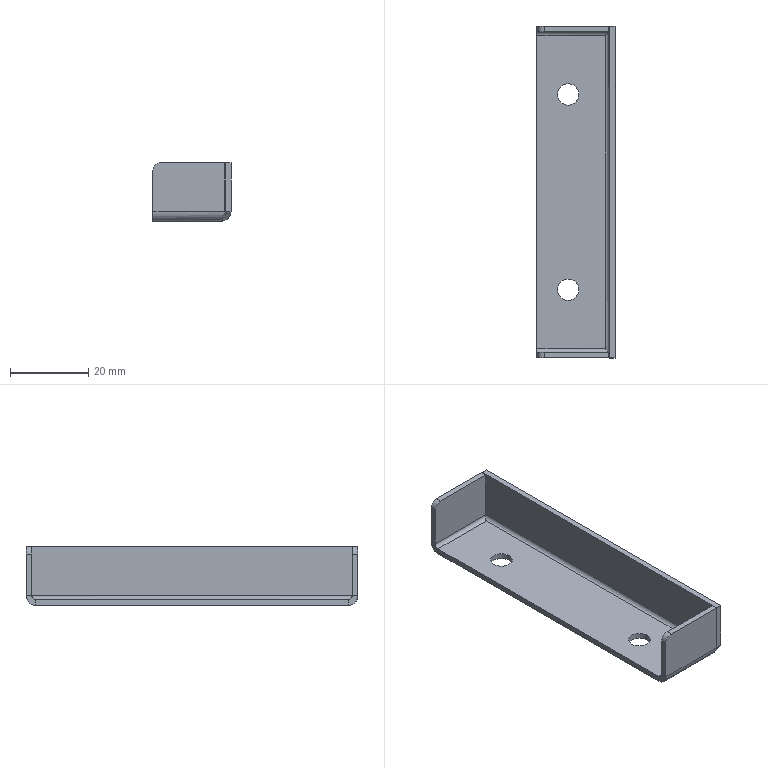Part | STEP file | FBDS-BJ-014 | 1 solid | 36 faces | box 20 x 85 x 15 mm | volume 4798 mm3 | plane 20 | cylinder 12 | spline 4 | commonest cylinder face diameters 5.5 x4 2 x3 5 x3 4 x2
STEP:
#1=CARTESIAN_POINT('',(0.75,-25.,0.));
#2=VERTEX_POINT('',#1);
#3=CARTESIAN_POINT('',(-4.75,-25.,0.));
#4=VERTEX_POINT('',#3);
#5=CARTESIAN_POINT('',(-2.,-25.,0.));
#6=DIRECTION('',(0.,0.,-1.));
#7=DIRECTION('',(-1.,0.,0.));
#8=AXIS2_PLACEMENT_3D('',#5,#6,#7);
#9=CIRCLE('',#8,2.75);
#10=EDGE_CURVE('',#2,#4,#9,.T.);
#11=ORIENTED_EDGE('',*,*,#10,.F.);
#12=CARTESIAN_POINT('',(0.75,-25.,-1.5));
#13=VERTEX_POINT('',#12);
#14=CARTESIAN_POINT('',(0.75,-25.,-1.5));
#15=DIRECTION('',(0.,0.,-1.));
#16=VECTOR('',#15,1000.);
#17=LINE('',#14,#16);
#18=EDGE_CURVE('',#2,#13,#17,.T.);
#19=ORIENTED_EDGE('',*,*,#18,.T.);
#20=CARTESIAN_POINT('',(-4.75,-25.,-1.5));
#21=VERTEX_POINT('',#20);
#22=CARTESIAN_POINT('',(-2.,-25.,-1.5));
#23=DIRECTION('',(0.,0.,-1.));
#24=DIRECTION('',(-1.,0.,0.));
#25=AXIS2_PLACEMENT_3D('',#22,#23,#24);
#26=CIRCLE('',#25,2.75);
#27=EDGE_CURVE('',#13,#21,#26,.T.);
#28=ORIENTED_EDGE('',*,*,#27,.T.);
#29=CARTESIAN_POINT('',(-4.75,-25.,-1.5));
#30=DIRECTION('',(0.,0.,-1.));
#31=VECTOR('',#30,1000.);
#32=LINE('',#29,#31);
#33=EDGE_CURVE('',#4,#21,#32,.T.);
#34=ORIENTED_EDGE('',*,*,#33,.F.);
#35=EDGE_LOOP('',(#11,#19,#28,#34));
#36=FACE_OUTER_BOUND('',#35,.T.);
#37=CARTESIAN_POINT('',(-2.,-25.,-1.5));
#38=DIRECTION('',(0.,0.,-1.));
#39=DIRECTION('',(-1.,0.,0.));
#40=AXIS2_PLACEMENT_3D('',#37,#38,#39);
#41=CYLINDRICAL_SURFACE('',#40,2.75);
#42=ADVANCED_FACE('',(#36),#41,.F.);
#43=CARTESIAN_POINT('',(0.75,25.,0.));
#44=VERTEX_POINT('',#43);
#45=CARTESIAN_POINT('',(-4.75,25.,0.));
#46=VERTEX_POINT('',#45);
#47=CARTESIAN_POINT('',(-2.,25.,0.));
#48=DIRECTION('',(0.,0.,-1.));
#49=DIRECTION('',(-1.,0.,0.));
#50=AXIS2_PLACEMENT_3D('',#47,#48,#49);
#51=CIRCLE('',#50,2.75);
#52=EDGE_CURVE('',#44,#46,#51,.T.);
#53=ORIENTED_EDGE('',*,*,#52,.F.);
#54=CARTESIAN_POINT('',(0.75,25.,-1.5));
#55=VERTEX_POINT('',#54);
#56=CARTESIAN_POINT('',(0.75,25.,-1.5));
#57=DIRECTION('',(0.,0.,-1.));
#58=VECTOR('',#57,1000.);
#59=LINE('',#56,#58);
#60=EDGE_CURVE('',#44,#55,#59,.T.);
#61=ORIENTED_EDGE('',*,*,#60,.T.);
#62=CARTESIAN_POINT('',(-4.75,25.,-1.5));
#63=VERTEX_POINT('',#62);
#64=CARTESIAN_POINT('',(-2.,25.,-1.5));
#65=DIRECTION('',(0.,0.,-1.));
#66=DIRECTION('',(-1.,0.,0.));
#67=AXIS2_PLACEMENT_3D('',#64,#65,#66);
#68=CIRCLE('',#67,2.75);
#69=EDGE_CURVE('',#55,#63,#68,.T.);
#70=ORIENTED_EDGE('',*,*,#69,.T.);
#71=CARTESIAN_POINT('',(-4.75,25.,-1.5));
#72=DIRECTION('',(0.,0.,-1.));
#73=VECTOR('',#72,1000.);
#74=LINE('',#71,#73);
#75=EDGE_CURVE('',#46,#63,#74,.T.);
#76=ORIENTED_EDGE('',*,*,#75,.F.);
#77=EDGE_LOOP('',(#53,#61,#70,#76));
#78=FACE_OUTER_BOUND('',#77,.T.);
#79=CARTESIAN_POINT('',(-2.,25.,-1.5));
#80=DIRECTION('',(0.,0.,-1.));
#81=DIRECTION('',(-1.,0.,0.));
#82=AXIS2_PLACEMENT_3D('',#79,#80,#81);
#83=CYLINDRICAL_SURFACE('',#82,2.75);
#84=ADVANCED_FACE('',(#78),#83,.F.);
#85=CARTESIAN_POINT('',(-2.,-25.,-1.5));
#86=DIRECTION('',(0.,0.,-1.));
#87=DIRECTION('',(-1.,0.,0.));
#88=AXIS2_PLACEMENT_3D('',#85,#86,#87);
#89=CIRCLE('',#88,2.75);
#90=EDGE_CURVE('',#21,#13,#89,.T.);
#91=ORIENTED_EDGE('',*,*,#90,.F.);
#92=ORIENTED_EDGE('',*,*,#27,.F.);
#93=EDGE_LOOP('',(#91,#92));
#94=FACE_BOUND('',#93,.T.);
#95=CARTESIAN_POINT('',(-2.,25.,-1.5));
#96=DIRECTION('',(0.,0.,-1.));
#97=DIRECTION('',(-1.,0.,0.));
#98=AXIS2_PLACEMENT_3D('',#95,#96,#97);
#99=CIRCLE('',#98,2.75);
#100=EDGE_CURVE('',#63,#55,#99,.T.);
#101=ORIENTED_EDGE('',*,*,#100,.F.);
#102=ORIENTED_EDGE('',*,*,#69,.F.);
#103=EDGE_LOOP('',(#101,#102));
#104=FACE_BOUND('',#103,.T.);
#105=CARTESIAN_POINT('',(7.5,40.,-1.5));
#106=VERTEX_POINT('',#105);
#107=CARTESIAN_POINT('',(-10.,40.,-1.5));
#108=VERTEX_POINT('',#107);
#109=CARTESIAN_POINT('',(10.,40.,-1.5));
#110=DIRECTION('',(-1.,0.,0.));
#111=VECTOR('',#110,1000.);
#112=LINE('',#109,#111);
#113=EDGE_CURVE('',#106,#108,#112,.T.);
#114=ORIENTED_EDGE('',*,*,#113,.F.);
#115=CARTESIAN_POINT('',(7.5,-40.,-1.5));
#116=VERTEX_POINT('',#115);
#117=CARTESIAN_POINT('',(7.5,40.,-1.5));
#118=DIRECTION('',(0.,-1.,0.));
#119=VECTOR('',#118,1000.);
#120=LINE('',#117,#119);
#121=EDGE_CURVE('',#106,#116,#120,.T.);
#122=ORIENTED_EDGE('',*,*,#121,.T.);
#123=CARTESIAN_POINT('',(-10.,-40.,-1.5));
#124=VERTEX_POINT('',#123);
#125=CARTESIAN_POINT('',(10.,-40.,-1.5));
#126=DIRECTION('',(1.,0.,0.));
#127=VECTOR('',#126,1000.);
#128=LINE('',#125,#127);
#129=EDGE_CURVE('',#124,#116,#128,.T.);
#130=ORIENTED_EDGE('',*,*,#129,.F.);
#131=CARTESIAN_POINT('',(-10.,40.,-1.5));
#132=DIRECTION('',(0.,-1.,0.));
#133=VECTOR('',#132,1000.);
#134=LINE('',#131,#133);
#135=EDGE_CURVE('',#108,#124,#134,.T.);
#136=ORIENTED_EDGE('',*,*,#135,.F.);
#137=EDGE_LOOP('',(#114,#122,#130,#136));
#138=FACE_OUTER_BOUND('',#137,.T.);
#139=CARTESIAN_POINT('',(0.,0.,-1.5));
#140=DIRECTION('',(0.,0.,-1.));
#141=DIRECTION('',(-1.,0.,0.));
#142=AXIS2_PLACEMENT_3D('',#139,#140,#141);
#143=PLANE('',#142);
#144=ADVANCED_FACE('',(#94,#104,#138),#143,.T.);
#145=CARTESIAN_POINT('',(-2.,-25.,0.));
#146=DIRECTION('',(0.,0.,-1.));
#147=DIRECTION('',(-1.,0.,0.));
#148=AXIS2_PLACEMENT_3D('',#145,#146,#147);
#149=CIRCLE('',#148,2.75);
#150=EDGE_CURVE('',#4,#2,#149,.T.);
#151=ORIENTED_EDGE('',*,*,#150,.T.);
#152=ORIENTED_EDGE('',*,*,#10,.T.);
#153=EDGE_LOOP('',(#151,#152));
#154=FACE_BOUND('',#153,.T.);
#155=CARTESIAN_POINT('',(-2.,25.,0.));
#156=DIRECTION('',(0.,0.,-1.));
#157=DIRECTION('',(-1.,0.,0.));
#158=AXIS2_PLACEMENT_3D('',#155,#156,#157);
#159=CIRCLE('',#158,2.75);
#160=EDGE_CURVE('',#46,#44,#159,.T.);
#161=ORIENTED_EDGE('',*,*,#160,.T.);
#162=ORIENTED_EDGE('',*,*,#52,.T.);
#163=EDGE_LOOP('',(#161,#162));
#164=FACE_BOUND('',#163,.T.);
#165=CARTESIAN_POINT('',(7.5,40.,0.));
#166=VERTEX_POINT('',#165);
#167=CARTESIAN_POINT('',(7.5,-40.,0.));
#168=VERTEX_POINT('',#167);
#169=CARTESIAN_POINT('',(7.5,40.,0.));
#170=DIRECTION('',(0.,-1.,0.));
#171=VECTOR('',#170,1000.);
#172=LINE('',#169,#171);
#173=EDGE_CURVE('',#166,#168,#172,.T.);
#174=ORIENTED_EDGE('',*,*,#173,.F.);
#175=CARTESIAN_POINT('',(-10.,40.,0.));
#176=VERTEX_POINT('',#175);
#177=CARTESIAN_POINT('',(10.,40.,0.));
#178=DIRECTION('',(-1.,0.,0.));
#179=VECTOR('',#178,1000.);
#180=LINE('',#177,#179);
#181=EDGE_CURVE('',#166,#176,#180,.T.);
#182=ORIENTED_EDGE('',*,*,#181,.T.);
#183=CARTESIAN_POINT('',(-10.,-40.,0.));
#184=VERTEX_POINT('',#183);
#185=CARTESIAN_POINT('',(-10.,40.,0.));
#186=DIRECTION('',(0.,-1.,0.));
#187=VECTOR('',#186,1000.);
#188=LINE('',#185,#187);
#189=EDGE_CURVE('',#176,#184,#188,.T.);
#190=ORIENTED_EDGE('',*,*,#189,.T.);
#191=CARTESIAN_POINT('',(10.,-40.,0.));
#192=DIRECTION('',(1.,0.,0.));
#193=VECTOR('',#192,1000.);
#194=LINE('',#191,#193);
#195=EDGE_CURVE('',#184,#168,#194,.T.);
#196=ORIENTED_EDGE('',*,*,#195,.T.);
#197=EDGE_LOOP('',(#174,#182,#190,#196));
#198=FACE_OUTER_BOUND('',#197,.T.);
#199=CARTESIAN_POINT('',(0.,0.,0.));
#200=DIRECTION('',(0.,0.,-1.));
#201=DIRECTION('',(-1.,0.,0.));
#202=AXIS2_PLACEMENT_3D('',#199,#200,#201);
#203=PLANE('',#202);
#204=ADVANCED_FACE('',(#154,#164,#198),#203,.F.);
#205=ORIENTED_EDGE('',*,*,#189,.F.);
#206=CARTESIAN_POINT('',(-10.,40.,-1.5));
#207=DIRECTION('',(0.,0.,1.));
#208=VECTOR('',#207,1000.);
#209=LINE('',#206,#208);
#210=EDGE_CURVE('',#108,#176,#209,.T.);
#211=ORIENTED_EDGE('',*,*,#210,.F.);
#212=ORIENTED_EDGE('',*,*,#135,.T.);
#213=CARTESIAN_POINT('',(-10.,-40.,-1.5));
#214=DIRECTION('',(0.,0.,1.));
#215=VECTOR('',#214,1000.);
#216=LINE('',#213,#215);
#217=EDGE_CURVE('',#124,#184,#216,.T.);
#218=ORIENTED_EDGE('',*,*,#217,.T.);
#219=EDGE_LOOP('',(#205,#211,#212,#218));
#220=FACE_OUTER_BOUND('',#219,.T.);
#221=CARTESIAN_POINT('',(-10.,40.,-1.5));
#222=DIRECTION('',(-1.,0.,0.));
#223=DIRECTION('',(0.,-1.,0.));
#224=AXIS2_PLACEMENT_3D('',#221,#222,#223);
#225=PLANE('',#224);
#226=ADVANCED_FACE('',(#220),#225,.T.);
#227=ORIENTED_EDGE('',*,*,#60,.F.);
#228=ORIENTED_EDGE('',*,*,#160,.F.);
#229=ORIENTED_EDGE('',*,*,#75,.T.);
#230=ORIENTED_EDGE('',*,*,#100,.T.);
#231=EDGE_LOOP('',(#227,#228,#229,#230));
#232=FACE_OUTER_BOUND('',#231,.T.);
#233=CARTESIAN_POINT('',(-2.,25.,-1.5));
#234=DIRECTION('',(0.,0.,-1.));
#235=DIRECTION('',(-1.,0.,0.));
#236=AXIS2_PLACEMENT_3D('',#233,#234,#235);
#237=CYLINDRICAL_SURFACE('',#236,2.75);
#238=ADVANCED_FACE('',(#232),#237,.F.);
#239=ORIENTED_EDGE('',*,*,#18,.F.);
#240=ORIENTED_EDGE('',*,*,#150,.F.);
#241=ORIENTED_EDGE('',*,*,#33,.T.);
#242=ORIENTED_EDGE('',*,*,#90,.T.);
#243=EDGE_LOOP('',(#239,#240,#241,#242));
#244=FACE_OUTER_BOUND('',#243,.T.);
#245=CARTESIAN_POINT('',(-2.,-25.,-1.5));
#246=DIRECTION('',(0.,0.,-1.));
#247=DIRECTION('',(-1.,0.,0.));
#248=AXIS2_PLACEMENT_3D('',#245,#246,#247);
#249=CYLINDRICAL_SURFACE('',#248,2.75);
#250=ADVANCED_FACE('',(#244),#249,.F.);
#251=CARTESIAN_POINT('',(-10.,-41.,1.));
#252=VERTEX_POINT('',#251);
#253=CARTESIAN_POINT('',(-10.,-42.5,1.));
#254=VERTEX_POINT('',#253);
#255=CARTESIAN_POINT('',(-10.,-42.5,1.));
#256=DIRECTION('',(0.,-1.,0.));
#257=VECTOR('',#256,1000.);
#258=LINE('',#255,#257);
#259=EDGE_CURVE('',#252,#254,#258,.T.);
#260=ORIENTED_EDGE('',*,*,#259,.F.);
#261=CARTESIAN_POINT('',(-10.,-40.,1.));
#262=DIRECTION('',(1.,0.,0.));
#263=DIRECTION('',(0.,-1.,0.));
#264=AXIS2_PLACEMENT_3D('',#261,#262,#263);
#265=CIRCLE('',#264,1.);
#266=EDGE_CURVE('',#252,#184,#265,.T.);
#267=ORIENTED_EDGE('',*,*,#266,.T.);
#268=ORIENTED_EDGE('',*,*,#217,.F.);
#269=CARTESIAN_POINT('',(-10.,-40.,1.));
#270=DIRECTION('',(1.,0.,0.));
#271=DIRECTION('',(0.,0.,-1.));
#272=AXIS2_PLACEMENT_3D('',#269,#270,#271);
#273=CIRCLE('',#272,2.5);
#274=EDGE_CURVE('',#254,#124,#273,.T.);
#275=ORIENTED_EDGE('',*,*,#274,.F.);
#276=EDGE_LOOP('',(#260,#267,#268,#275));
#277=FACE_OUTER_BOUND('',#276,.T.);
#278=CARTESIAN_POINT('',(-10.,-40.,1.));
#279=DIRECTION('',(-1.,0.,0.));
#280=DIRECTION('',(0.,0.,1.));
#281=AXIS2_PLACEMENT_3D('',#278,#279,#280);
#282=PLANE('',#281);
#283=ADVANCED_FACE('',(#277),#282,.T.);
#284=CARTESIAN_POINT('',(8.4,-41.,1.));
#285=VERTEX_POINT('',#284);
#286=CARTESIAN_POINT('',(7.5,-40.,0.));
#287=CARTESIAN_POINT('',(7.576,-40.132,0.));
#288=CARTESIAN_POINT('',(7.649,-40.26,0.02555));
#289=CARTESIAN_POINT('',(7.799,-40.503,0.1256));
#290=CARTESIAN_POINT('',(7.874,-40.613,0.1992));
#291=CARTESIAN_POINT('',(8.025,-40.799,0.3847));
#292=CARTESIAN_POINT('',(8.099,-40.873,0.4949));
#293=CARTESIAN_POINT('',(8.25,-40.974,0.7376));
#294=CARTESIAN_POINT('',(8.324,-41.,0.8678));
#295=CARTESIAN_POINT('',(8.4,-41.,1.));
#296=B_SPLINE_CURVE_WITH_KNOTS('',3,(#286,#287,#288,#289,#290,#291,#292,#293,#294,#295),.UNSPECIFIED.,.F.,.F.,(4,2,2,2,4),(0.,0.0004487,0.0008973,0.001346,0.001795),.UNSPECIFIED.);
#297=EDGE_CURVE('',#168,#285,#296,.T.);
#298=ORIENTED_EDGE('',*,*,#297,.T.);
#299=CARTESIAN_POINT('',(8.4,-42.5,1.));
#300=VERTEX_POINT('',#299);
#301=CARTESIAN_POINT('',(8.4,-41.,1.));
#302=CARTESIAN_POINT('',(8.4,-42.5,1.));
#303=B_SPLINE_CURVE_WITH_KNOTS('',1,(#301,#302),.UNSPECIFIED.,.F.,.F.,(2,2),(0.,1.),.UNSPECIFIED.);
#304=EDGE_CURVE('',#285,#300,#303,.T.);
#305=ORIENTED_EDGE('',*,*,#304,.T.);
#306=CARTESIAN_POINT('',(7.5,-40.,-1.5));
#307=CARTESIAN_POINT('',(7.538,-40.165,-1.5));
#308=CARTESIAN_POINT('',(7.575,-40.328,-1.484));
#309=CARTESIAN_POINT('',(7.65,-40.648,-1.42));
#310=CARTESIAN_POINT('',(7.688,-40.807,-1.372));
#311=CARTESIAN_POINT('',(7.763,-41.109,-1.247));
#312=CARTESIAN_POINT('',(7.8,-41.252,-1.17));
#313=CARTESIAN_POINT('',(7.875,-41.524,-0.9883));
#314=CARTESIAN_POINT('',(7.913,-41.652,-0.883));
#315=CARTESIAN_POINT('',(8.025,-41.998,-0.5378));
#316=CARTESIAN_POINT('',(8.1,-42.184,-0.259));
#317=CARTESIAN_POINT('',(8.249,-42.434,0.3419));
#318=CARTESIAN_POINT('',(8.324,-42.5,0.67));
#319=CARTESIAN_POINT('',(8.4,-42.5,1.));
#320=B_SPLINE_CURVE_WITH_KNOTS('',3,(#306,#307,#308,#309,#310,#311,#312,#313,#314,#315,#316,#317,#318,#319),.UNSPECIFIED.,.F.,.F.,(4,2,2,2,2,2,4),(0.,0.0005023,0.001005,0.001507,0.002009,0.003014,0.004019),.UNSPECIFIED.);
#321=EDGE_CURVE('',#116,#300,#320,.T.);
#322=ORIENTED_EDGE('',*,*,#321,.F.);
#323=CARTESIAN_POINT('',(7.5,-40.,0.));
#324=CARTESIAN_POINT('',(7.5,-40.,-1.5));
#325=B_SPLINE_CURVE_WITH_KNOTS('',1,(#323,#324),.UNSPECIFIED.,.F.,.F.,(2,2),(0.,1.),.UNSPECIFIED.);
#326=EDGE_CURVE('',#168,#116,#325,.T.);
#327=ORIENTED_EDGE('',*,*,#326,.F.);
#328=EDGE_LOOP('',(#298,#305,#322,#327));
#329=FACE_OUTER_BOUND('',#328,.T.);
#330=CARTESIAN_POINT('',(7.5,-40.,-1.515));
#331=CARTESIAN_POINT('',(7.575,-40.329,-1.515));
#332=CARTESIAN_POINT('',(7.65,-40.658,-1.45));
#333=CARTESIAN_POINT('',(7.8,-41.267,-1.198));
#334=CARTESIAN_POINT('',(7.875,-41.546,-1.011));
#335=CARTESIAN_POINT('',(8.025,-42.011,-0.5457));
#336=CARTESIAN_POINT('',(8.1,-42.198,-0.2667));
#337=CARTESIAN_POINT('',(8.25,-42.45,0.3417));
#338=CARTESIAN_POINT('',(8.325,-42.515,0.6707));
#339=CARTESIAN_POINT('',(8.4,-42.515,1.));
#340=CARTESIAN_POINT('',(7.5,-40.,-1.5));
#341=CARTESIAN_POINT('',(7.575,-40.327,-1.5));
#342=CARTESIAN_POINT('',(7.65,-40.654,-1.435));
#343=CARTESIAN_POINT('',(7.8,-41.259,-1.184));
#344=CARTESIAN_POINT('',(7.875,-41.536,-0.9992));
#345=CARTESIAN_POINT('',(8.025,-41.999,-0.5364));
#346=CARTESIAN_POINT('',(8.1,-42.184,-0.259));
#347=CARTESIAN_POINT('',(8.25,-42.435,0.3456));
#348=CARTESIAN_POINT('',(8.325,-42.5,0.6727));
#349=CARTESIAN_POINT('',(8.4,-42.5,1.));
#350=CARTESIAN_POINT('',(7.5,-40.,0.));
#351=CARTESIAN_POINT('',(7.575,-40.131,0.));
#352=CARTESIAN_POINT('',(7.65,-40.262,0.02603));
#353=CARTESIAN_POINT('',(7.8,-40.504,0.1262));
#354=CARTESIAN_POINT('',(7.875,-40.615,0.2003));
#355=CARTESIAN_POINT('',(8.025,-40.8,0.3855));
#356=CARTESIAN_POINT('',(8.1,-40.874,0.4964));
#357=CARTESIAN_POINT('',(8.25,-40.974,0.7383));
#358=CARTESIAN_POINT('',(8.325,-41.,0.8691));
#359=CARTESIAN_POINT('',(8.4,-41.,1.));
#360=CARTESIAN_POINT('',(7.5,-40.,0.015));
#361=CARTESIAN_POINT('',(7.575,-40.129,0.015));
#362=CARTESIAN_POINT('',(7.65,-40.258,0.04064));
#363=CARTESIAN_POINT('',(7.8,-40.496,0.1393));
#364=CARTESIAN_POINT('',(7.875,-40.605,0.2123));
#365=CARTESIAN_POINT('',(8.025,-40.788,0.3947));
#366=CARTESIAN_POINT('',(8.1,-40.861,0.5039));
#367=CARTESIAN_POINT('',(8.25,-40.959,0.7422));
#368=CARTESIAN_POINT('',(8.325,-40.985,0.871));
#369=CARTESIAN_POINT('',(8.4,-40.985,1.));
#370=B_SPLINE_SURFACE_WITH_KNOTS('',1,3,((#330,#331,#332,#333,#334,#335,#336,#337,#338,#339),(#340,#341,#342,#343,#344,#345,#346,#347,#348,#349),(#350,#351,#352,#353,#354,#355,#356,#357,#358,#359),(#360,#361,#362,#363,#364,#365,#366,#367,#368,#369)),.UNSPECIFIED.,.F.,.F.,.F.,(2,1,1,2),(4,2,2,2,4),(-0.0101,0.,1.,1.01),(0.,0.25,0.5,0.75,1.),.UNSPECIFIED.);
#371=ADVANCED_FACE('',(#329),#370,.T.);
#372=ORIENTED_EDGE('',*,*,#129,.T.);
#373=ORIENTED_EDGE('',*,*,#321,.T.);
#374=CARTESIAN_POINT('',(-10.,-42.5,1.));
#375=DIRECTION('',(-1.,0.,0.));
#376=VECTOR('',#375,1000.);
#377=LINE('',#374,#376);
#378=EDGE_CURVE('',#300,#254,#377,.T.);
#379=ORIENTED_EDGE('',*,*,#378,.T.);
#380=ORIENTED_EDGE('',*,*,#274,.T.);
#381=EDGE_LOOP('',(#372,#373,#379,#380));
#382=FACE_OUTER_BOUND('',#381,.T.);
#383=CARTESIAN_POINT('',(17.415,-40.,1.));
#384=DIRECTION('',(-1.,0.,0.));
#385=DIRECTION('',(0.,-1.,0.));
#386=AXIS2_PLACEMENT_3D('',#383,#384,#385);
#387=CYLINDRICAL_SURFACE('',#386,2.5);
#388=ADVANCED_FACE('',(#382),#387,.T.);
#389=ORIENTED_EDGE('',*,*,#195,.F.);
#390=ORIENTED_EDGE('',*,*,#266,.F.);
#391=CARTESIAN_POINT('',(-10.,-41.,1.));
#392=DIRECTION('',(1.,0.,0.));
#393=VECTOR('',#392,1000.);
#394=LINE('',#391,#393);
#395=EDGE_CURVE('',#252,#285,#394,.T.);
#396=ORIENTED_EDGE('',*,*,#395,.T.);
#397=ORIENTED_EDGE('',*,*,#297,.F.);
#398=EDGE_LOOP('',(#389,#390,#396,#397));
#399=FACE_OUTER_BOUND('',#398,.T.);
#400=CARTESIAN_POINT('',(17.415,-40.,1.));
#401=DIRECTION('',(-1.,0.,0.));
#402=DIRECTION('',(0.,-1.,0.));
#403=AXIS2_PLACEMENT_3D('',#400,#401,#402);
#404=CYLINDRICAL_SURFACE('',#403,1.);
#405=ADVANCED_FACE('',(#399),#404,.F.);
#406=CARTESIAN_POINT('',(-8.,-42.5,13.5));
#407=VERTEX_POINT('',#406);
#408=CARTESIAN_POINT('',(-10.,-42.5,11.5));
#409=VERTEX_POINT('',#408);
#410=CARTESIAN_POINT('',(-8.,-42.5,11.5));
#411=DIRECTION('',(0.,-1.,0.));
#412=DIRECTION('',(0.,0.,1.));
#413=AXIS2_PLACEMENT_3D('',#410,#411,#412);
#414=CIRCLE('',#413,2.);
#415=EDGE_CURVE('',#407,#409,#414,.T.);
#416=ORIENTED_EDGE('',*,*,#415,.F.);
#417=CARTESIAN_POINT('',(-8.,-41.,13.5));
#418=VERTEX_POINT('',#417);
#419=CARTESIAN_POINT('',(-8.,-42.5,13.5));
#420=DIRECTION('',(0.,-1.,0.));
#421=VECTOR('',#420,1000.);
#422=LINE('',#419,#421);
#423=EDGE_CURVE('',#418,#407,#422,.T.);
#424=ORIENTED_EDGE('',*,*,#423,.F.);
#425=CARTESIAN_POINT('',(-10.,-41.,11.5));
#426=VERTEX_POINT('',#425);
#427=CARTESIAN_POINT('',(-8.,-41.,11.5));
#428=DIRECTION('',(0.,1.,0.));
#429=DIRECTION('',(0.,0.,1.));
#430=AXIS2_PLACEMENT_3D('',#427,#428,#429);
#431=CIRCLE('',#430,2.);
#432=EDGE_CURVE('',#426,#418,#431,.T.);
#433=ORIENTED_EDGE('',*,*,#432,.F.);
#434=CARTESIAN_POINT('',(-10.,-42.5,11.5));
#435=DIRECTION('',(0.,1.,0.));
#436=VECTOR('',#435,1000.);
#437=LINE('',#434,#436);
#438=EDGE_CURVE('',#409,#426,#437,.T.);
#439=ORIENTED_EDGE('',*,*,#438,.F.);
#440=EDGE_LOOP('',(#416,#424,#433,#439));
#441=FACE_OUTER_BOUND('',#440,.T.);
#442=CARTESIAN_POINT('',(-8.,-42.5,11.5));
#443=DIRECTION('',(0.,1.,0.));
#444=DIRECTION('',(0.,0.,1.));
#445=AXIS2_PLACEMENT_3D('',#442,#443,#444);
#446=CYLINDRICAL_SURFACE('',#445,2.);
#447=ADVANCED_FACE('',(#441),#446,.T.);
#448=CARTESIAN_POINT('',(8.4,-41.,13.5));
#449=VERTEX_POINT('',#448);
#450=CARTESIAN_POINT('',(-10.,-41.,13.5));
#451=DIRECTION('',(-1.,0.,0.));
#452=VECTOR('',#451,1000.);
#453=LINE('',#450,#452);
#454=EDGE_CURVE('',#449,#418,#453,.T.);
#455=ORIENTED_EDGE('',*,*,#454,.T.);
#456=ORIENTED_EDGE('',*,*,#423,.T.);
#457=CARTESIAN_POINT('',(8.4,-42.5,13.5));
#458=VERTEX_POINT('',#457);
#459=CARTESIAN_POINT('',(0.,-42.5,13.5));
#460=DIRECTION('',(-1.,0.,0.));
#461=VECTOR('',#460,1000.);
#462=LINE('',#459,#461);
#463=EDGE_CURVE('',#458,#407,#462,.T.);
#464=ORIENTED_EDGE('',*,*,#463,.F.);
#465=CARTESIAN_POINT('',(8.4,-41.,13.5));
#466=DIRECTION('',(0.,-1.,0.));
#467=VECTOR('',#466,1000.);
#468=LINE('',#465,#467);
#469=EDGE_CURVE('',#449,#458,#468,.T.);
#470=ORIENTED_EDGE('',*,*,#469,.F.);
#471=EDGE_LOOP('',(#455,#456,#464,#470));
#472=FACE_OUTER_BOUND('',#471,.T.);
#473=CARTESIAN_POINT('',(-10.,-42.5,13.5));
#474=DIRECTION('',(0.,0.,-1.));
#475=DIRECTION('',(0.,1.,0.));
#476=AXIS2_PLACEMENT_3D('',#473,#474,#475);
#477=PLANE('',#476);
#478=ADVANCED_FACE('',(#472),#477,.F.);
#479=ORIENTED_EDGE('',*,*,#463,.T.);
#480=ORIENTED_EDGE('',*,*,#415,.T.);
#481=CARTESIAN_POINT('',(-10.,-42.5,0.));
#482=DIRECTION('',(0.,0.,-1.));
#483=VECTOR('',#482,1000.);
#484=LINE('',#481,#483);
#485=EDGE_CURVE('',#409,#254,#484,.T.);
#486=ORIENTED_EDGE('',*,*,#485,.T.);
#487=ORIENTED_EDGE('',*,*,#378,.F.);
#488=CARTESIAN_POINT('',(8.4,-42.5,1.));
#489=DIRECTION('',(0.,0.,1.));
#490=VECTOR('',#489,1000.);
#491=LINE('',#488,#490);
#492=EDGE_CURVE('',#300,#458,#491,.T.);
#493=ORIENTED_EDGE('',*,*,#492,.T.);
#494=EDGE_LOOP('',(#479,#480,#486,#487,#493));
#495=FACE_OUTER_BOUND('',#494,.T.);
#496=CARTESIAN_POINT('',(0.,-42.5,0.));
#497=DIRECTION('',(0.,1.,0.));
#498=DIRECTION('',(0.,0.,1.));
#499=AXIS2_PLACEMENT_3D('',#496,#497,#498);
#500=PLANE('',#499);
#501=ADVANCED_FACE('',(#495),#500,.F.);
#502=ORIENTED_EDGE('',*,*,#492,.F.);
#503=ORIENTED_EDGE('',*,*,#304,.F.);
#504=CARTESIAN_POINT('',(8.4,-41.,1.));
#505=DIRECTION('',(0.,0.,1.));
#506=VECTOR('',#505,1000.);
#507=LINE('',#504,#506);
#508=EDGE_CURVE('',#285,#449,#507,.T.);
#509=ORIENTED_EDGE('',*,*,#508,.T.);
#510=ORIENTED_EDGE('',*,*,#469,.T.);
#511=EDGE_LOOP('',(#502,#503,#509,#510));
#512=FACE_OUTER_BOUND('',#511,.T.);
#513=CARTESIAN_POINT('',(8.4,-41.,1.));
#514=DIRECTION('',(1.,0.,0.));
#515=DIRECTION('',(0.,-1.,0.));
#516=AXIS2_PLACEMENT_3D('',#513,#514,#515);
#517=PLANE('',#516);
#518=ADVANCED_FACE('',(#512),#517,.T.);
#519=CARTESIAN_POINT('',(-10.,-41.,0.));
#520=DIRECTION('',(0.,0.,-1.));
#521=VECTOR('',#520,1000.);
#522=LINE('',#519,#521);
#523=EDGE_CURVE('',#426,#252,#522,.T.);
#524=ORIENTED_EDGE('',*,*,#523,.F.);
#525=ORIENTED_EDGE('',*,*,#432,.T.);
#526=ORIENTED_EDGE('',*,*,#454,.F.);
#527=ORIENTED_EDGE('',*,*,#508,.F.);
#528=ORIENTED_EDGE('',*,*,#395,.F.);
#529=EDGE_LOOP('',(#524,#525,#526,#527,#528));
#530=FACE_OUTER_BOUND('',#529,.T.);
#531=CARTESIAN_POINT('',(0.,-41.,0.));
#532=DIRECTION('',(0.,1.,0.));
#533=DIRECTION('',(0.,0.,1.));
#534=AXIS2_PLACEMENT_3D('',#531,#532,#533);
#535=PLANE('',#534);
#536=ADVANCED_FACE('',(#530),#535,.T.);
#537=ORIENTED_EDGE('',*,*,#485,.F.);
#538=ORIENTED_EDGE('',*,*,#438,.T.);
#539=ORIENTED_EDGE('',*,*,#523,.T.);
#540=ORIENTED_EDGE('',*,*,#259,.T.);
#541=EDGE_LOOP('',(#537,#538,#539,#540));
#542=FACE_OUTER_BOUND('',#541,.T.);
#543=CARTESIAN_POINT('',(-10.,-42.5,0.));
#544=DIRECTION('',(1.,0.,0.));
#545=DIRECTION('',(0.,0.,-1.));
#546=AXIS2_PLACEMENT_3D('',#543,#544,#545);
#547=PLANE('',#546);
#548=ADVANCED_FACE('',(#542),#547,.F.);
#549=CARTESIAN_POINT('',(8.5,-42.5,13.5));
#550=VERTEX_POINT('',#549);
#551=CARTESIAN_POINT('',(8.5,42.5,13.5));
#552=VERTEX_POINT('',#551);
#553=CARTESIAN_POINT('',(8.5,0.,13.5));
#554=DIRECTION('',(0.,1.,0.));
#555=VECTOR('',#554,1000.);
#556=LINE('',#553,#555);
#557=EDGE_CURVE('',#550,#552,#556,.T.);
#558=ORIENTED_EDGE('',*,*,#557,.F.);
#559=CARTESIAN_POINT('',(10.,-42.5,13.5));
#560=VERTEX_POINT('',#559);
#561=CARTESIAN_POINT('',(10.,-42.5,13.5));
#562=DIRECTION('',(-1.,0.,0.));
#563=VECTOR('',#562,1000.);
#564=LINE('',#561,#563);
#565=EDGE_CURVE('',#560,#550,#564,.T.);
#566=ORIENTED_EDGE('',*,*,#565,.F.);
#567=CARTESIAN_POINT('',(10.,42.5,13.5));
#568=VERTEX_POINT('',#567);
#569=CARTESIAN_POINT('',(10.,40.,13.5));
#570=DIRECTION('',(0.,1.,0.));
#571=VECTOR('',#570,1000.);
#572=LINE('',#569,#571);
#573=EDGE_CURVE('',#560,#568,#572,.T.);
#574=ORIENTED_EDGE('',*,*,#573,.T.);
#575=CARTESIAN_POINT('',(10.,42.5,13.5));
#576=DIRECTION('',(-1.,0.,0.));
#577=VECTOR('',#576,1000.);
#578=LINE('',#575,#577);
#579=EDGE_CURVE('',#568,#552,#578,.T.);
#580=ORIENTED_EDGE('',*,*,#579,.T.);
#581=EDGE_LOOP('',(#558,#566,#574,#580));
#582=FACE_OUTER_BOUND('',#581,.T.);
#583=CARTESIAN_POINT('',(10.,40.,13.5));
#584=DIRECTION('',(0.,0.,1.));
#585=DIRECTION('',(1.,0.,0.));
#586=AXIS2_PLACEMENT_3D('',#583,#584,#585);
#587=PLANE('',#586);
#588=ADVANCED_FACE('',(#582),#587,.T.);
#589=ORIENTED_EDGE('',*,*,#573,.F.);
#590=CARTESIAN_POINT('',(10.,-42.5,1.));
#591=VERTEX_POINT('',#590);
#592=CARTESIAN_POINT('',(10.,-42.5,1.));
#593=DIRECTION('',(0.,0.,1.));
#594=VECTOR('',#593,1000.);
#595=LINE('',#592,#594);
#596=EDGE_CURVE('',#591,#560,#595,.T.);
#597=ORIENTED_EDGE('',*,*,#596,.F.);
#598=CARTESIAN_POINT('',(10.,42.5,1.));
#599=VERTEX_POINT('',#598);
#600=CARTESIAN_POINT('',(10.,0.,1.));
#601=DIRECTION('',(0.,1.,0.));
#602=VECTOR('',#601,1000.);
#603=LINE('',#600,#602);
#604=EDGE_CURVE('',#591,#599,#603,.T.);
#605=ORIENTED_EDGE('',*,*,#604,.T.);
#606=CARTESIAN_POINT('',(10.,42.5,1.));
#607=DIRECTION('',(0.,0.,1.));
#608=VECTOR('',#607,1000.);
#609=LINE('',#606,#608);
#610=EDGE_CURVE('',#599,#568,#609,.T.);
#611=ORIENTED_EDGE('',*,*,#610,.T.);
#612=EDGE_LOOP('',(#589,#597,#605,#611));
#613=FACE_OUTER_BOUND('',#612,.T.);
#614=CARTESIAN_POINT('',(10.,0.,0.));
#615=DIRECTION('',(1.,0.,0.));
#616=DIRECTION('',(0.,0.,-1.));
#617=AXIS2_PLACEMENT_3D('',#614,#615,#616);
#618=PLANE('',#617);
#619=ADVANCED_FACE('',(#613),#618,.T.);
#620=CARTESIAN_POINT('',(8.5,42.5,1.));
#621=VERTEX_POINT('',#620);
#622=CARTESIAN_POINT('',(8.5,42.5,1.));
#623=DIRECTION('',(0.,0.,1.));
#624=VECTOR('',#623,1000.);
#625=LINE('',#622,#624);
#626=EDGE_CURVE('',#621,#552,#625,.T.);
#627=ORIENTED_EDGE('',*,*,#626,.T.);
#628=ORIENTED_EDGE('',*,*,#579,.F.);
#629=ORIENTED_EDGE('',*,*,#610,.F.);
#630=CARTESIAN_POINT('',(10.,42.5,1.));
#631=CARTESIAN_POINT('',(9.5,42.5,1.));
#632=CARTESIAN_POINT('',(9.,42.5,1.));
#633=CARTESIAN_POINT('',(8.5,42.5,1.));
#634=B_SPLINE_CURVE_WITH_KNOTS('',3,(#630,#631,#632,#633),.UNSPECIFIED.,.F.,.F.,(4,4),(0.,1.),.UNSPECIFIED.);
#635=EDGE_CURVE('',#599,#621,#634,.T.);
#636=ORIENTED_EDGE('',*,*,#635,.T.);
#637=EDGE_LOOP('',(#627,#628,#629,#636));
#638=FACE_OUTER_BOUND('',#637,.T.);
#639=CARTESIAN_POINT('',(10.,42.5,1.));
#640=DIRECTION('',(0.,-1.,0.));
#641=DIRECTION('',(0.,0.,-1.));
#642=AXIS2_PLACEMENT_3D('',#639,#640,#641);
#643=PLANE('',#642);
#644=ADVANCED_FACE('',(#638),#643,.F.);
#645=CARTESIAN_POINT('',(8.5,-42.5,1.));
#646=VERTEX_POINT('',#645);
#647=CARTESIAN_POINT('',(8.5,-40.,1.));
#648=DIRECTION('',(0.,1.,0.));
#649=VECTOR('',#648,1000.);
#650=LINE('',#647,#649);
#651=EDGE_CURVE('',#646,#621,#650,.T.);
#652=ORIENTED_EDGE('',*,*,#651,.F.);
#653=CARTESIAN_POINT('',(8.5,-42.5,1.));
#654=DIRECTION('',(0.,0.,1.));
#655=VECTOR('',#654,1000.);
#656=LINE('',#653,#655);
#657=EDGE_CURVE('',#646,#550,#656,.T.);
#658=ORIENTED_EDGE('',*,*,#657,.T.);
#659=ORIENTED_EDGE('',*,*,#557,.T.);
#660=ORIENTED_EDGE('',*,*,#626,.F.);
#661=EDGE_LOOP('',(#652,#658,#659,#660));
#662=FACE_OUTER_BOUND('',#661,.T.);
#663=CARTESIAN_POINT('',(8.5,0.,0.));
#664=DIRECTION('',(1.,0.,0.));
#665=DIRECTION('',(0.,0.,-1.));
#666=AXIS2_PLACEMENT_3D('',#663,#664,#665);
#667=PLANE('',#666);
#668=ADVANCED_FACE('',(#662),#667,.F.);
#669=ORIENTED_EDGE('',*,*,#657,.F.);
#670=CARTESIAN_POINT('',(8.5,-42.5,1.));
#671=CARTESIAN_POINT('',(9.,-42.5,1.));
#672=CARTESIAN_POINT('',(9.5,-42.5,1.));
#673=CARTESIAN_POINT('',(10.,-42.5,1.));
#674=B_SPLINE_CURVE_WITH_KNOTS('',3,(#670,#671,#672,#673),.UNSPECIFIED.,.F.,.F.,(4,4),(0.,1.),.UNSPECIFIED.);
#675=EDGE_CURVE('',#646,#591,#674,.T.);
#676=ORIENTED_EDGE('',*,*,#675,.T.);
#677=ORIENTED_EDGE('',*,*,#596,.T.);
#678=ORIENTED_EDGE('',*,*,#565,.T.);
#679=EDGE_LOOP('',(#669,#676,#677,#678));
#680=FACE_OUTER_BOUND('',#679,.T.);
#681=CARTESIAN_POINT('',(10.,-42.5,1.));
#682=DIRECTION('',(0.,-1.,0.));
#683=DIRECTION('',(0.,0.,-1.));
#684=AXIS2_PLACEMENT_3D('',#681,#682,#683);
#685=PLANE('',#684);
#686=ADVANCED_FACE('',(#680),#685,.T.);
#687=ORIENTED_EDGE('',*,*,#675,.F.);
#688=CARTESIAN_POINT('',(8.5,-42.5,1.));
#689=CARTESIAN_POINT('',(8.5,-42.292,0.8691));
#690=CARTESIAN_POINT('',(8.474,-42.083,0.7383));
#691=CARTESIAN_POINT('',(8.374,-41.667,0.4964));
#692=CARTESIAN_POINT('',(8.3,-41.458,0.3855));
#693=CARTESIAN_POINT('',(8.115,-41.042,0.2003));
#694=CARTESIAN_POINT('',(8.004,-40.833,0.1262));
#695=CARTESIAN_POINT('',(7.762,-40.417,0.02603));
#696=CARTESIAN_POINT('',(7.631,-40.208,0.));
#697=CARTESIAN_POINT('',(7.5,-40.,0.));
#698=B_SPLINE_CURVE_WITH_KNOTS('',3,(#688,#689,#690,#691,#692,#693,#694,#695,#696,#697),.UNSPECIFIED.,.F.,.F.,(4,2,2,2,4),(0.,0.25,0.5,0.75,1.),.UNSPECIFIED.);
#699=EDGE_CURVE('',#646,#168,#698,.T.);
#700=ORIENTED_EDGE('',*,*,#699,.T.);
#701=ORIENTED_EDGE('',*,*,#326,.T.);
#702=CARTESIAN_POINT('',(10.,-42.5,1.));
#703=CARTESIAN_POINT('',(10.,-42.292,0.6728));
#704=CARTESIAN_POINT('',(9.935,-42.083,0.3456));
#705=CARTESIAN_POINT('',(9.684,-41.667,-0.259));
#706=CARTESIAN_POINT('',(9.499,-41.458,-0.5364));
#707=CARTESIAN_POINT('',(9.036,-41.042,-0.9992));
#708=CARTESIAN_POINT('',(8.759,-40.833,-1.184));
#709=CARTESIAN_POINT('',(8.154,-40.417,-1.435));
#710=CARTESIAN_POINT('',(7.827,-40.208,-1.5));
#711=CARTESIAN_POINT('',(7.5,-40.,-1.5));
#712=B_SPLINE_CURVE_WITH_KNOTS('',3,(#702,#703,#704,#705,#706,#707,#708,#709,#710,#711),.UNSPECIFIED.,.F.,.F.,(4,2,2,2,4),(0.,0.25,0.5,0.75,1.),.UNSPECIFIED.);
#713=EDGE_CURVE('',#591,#116,#712,.T.);
#714=ORIENTED_EDGE('',*,*,#713,.F.);
#715=EDGE_LOOP('',(#687,#700,#701,#714));
#716=FACE_OUTER_BOUND('',#715,.T.);
#717=CARTESIAN_POINT('',(10.,-42.5,1.));
#718=CARTESIAN_POINT('',(10.,-42.292,0.6727));
#719=CARTESIAN_POINT('',(9.935,-42.083,0.3456));
#720=CARTESIAN_POINT('',(9.684,-41.667,-0.259));
#721=CARTESIAN_POINT('',(9.499,-41.458,-0.5364));
#722=CARTESIAN_POINT('',(9.036,-41.042,-0.9992));
#723=CARTESIAN_POINT('',(8.759,-40.833,-1.184));
#724=CARTESIAN_POINT('',(8.154,-40.417,-1.435));
#725=CARTESIAN_POINT('',(7.827,-40.208,-1.5));
#726=CARTESIAN_POINT('',(7.5,-40.,-1.5));
#727=CARTESIAN_POINT('',(8.5,-42.5,1.));
#728=CARTESIAN_POINT('',(8.5,-42.292,0.8691));
#729=CARTESIAN_POINT('',(8.474,-42.083,0.7383));
#730=CARTESIAN_POINT('',(8.374,-41.667,0.4964));
#731=CARTESIAN_POINT('',(8.3,-41.458,0.3855));
#732=CARTESIAN_POINT('',(8.115,-41.042,0.2003));
#733=CARTESIAN_POINT('',(8.004,-40.833,0.1262));
#734=CARTESIAN_POINT('',(7.762,-40.417,0.02603));
#735=CARTESIAN_POINT('',(7.631,-40.208,0.));
#736=CARTESIAN_POINT('',(7.5,-40.,0.));
#737=B_SPLINE_SURFACE_WITH_KNOTS('',1,3,((#717,#718,#719,#720,#721,#722,#723,#724,#725,#726),(#727,#728,#729,#730,#731,#732,#733,#734,#735,#736)),.UNSPECIFIED.,.F.,.F.,.F.,(2,2),(4,2,2,2,4),(0.,1.),(0.,0.25,0.5,0.75,1.),.UNSPECIFIED.);
#738=ADVANCED_FACE('',(#716),#737,.T.);
#739=CARTESIAN_POINT('',(7.5,40.,0.));
#740=CARTESIAN_POINT('',(7.632,40.21,0.));
#741=CARTESIAN_POINT('',(7.762,40.417,0.02602));
#742=CARTESIAN_POINT('',(8.003,40.833,0.1261));
#743=CARTESIAN_POINT('',(8.115,41.043,0.2009));
#744=CARTESIAN_POINT('',(8.299,41.457,0.3848));
#745=CARTESIAN_POINT('',(8.373,41.663,0.4943));
#746=CARTESIAN_POINT('',(8.474,42.083,0.7378));
#747=CARTESIAN_POINT('',(8.5,42.29,0.8682));
#748=CARTESIAN_POINT('',(8.5,42.5,1.));
#749=B_SPLINE_CURVE_WITH_KNOTS('',3,(#739,#740,#741,#742,#743,#744,#745,#746,#747,#748),.UNSPECIFIED.,.F.,.F.,(4,2,2,2,4),(0.,0.0007358,0.001472,0.002208,0.002943),.UNSPECIFIED.);
#750=EDGE_CURVE('',#166,#621,#749,.T.);
#751=ORIENTED_EDGE('',*,*,#750,.T.);
#752=ORIENTED_EDGE('',*,*,#635,.F.);
#753=CARTESIAN_POINT('',(7.5,40.,-1.5));
#754=CARTESIAN_POINT('',(7.83,40.21,-1.5));
#755=CARTESIAN_POINT('',(8.151,40.415,-1.436));
#756=CARTESIAN_POINT('',(8.761,40.835,-1.184));
#757=CARTESIAN_POINT('',(9.034,41.04,-1.001));
#758=CARTESIAN_POINT('',(9.5,41.459,-0.5355));
#759=CARTESIAN_POINT('',(9.683,41.664,-0.2621));
#760=CARTESIAN_POINT('',(9.935,42.084,0.3461));
#761=CARTESIAN_POINT('',(10.,42.29,0.6697));
#762=CARTESIAN_POINT('',(10.,42.5,1.));
#763=B_SPLINE_CURVE_WITH_KNOTS('',3,(#753,#754,#755,#756,#757,#758,#759,#760,#761,#762),.UNSPECIFIED.,.F.,.F.,(4,2,2,2,4),(0.,0.001158,0.002316,0.003474,0.004632),.UNSPECIFIED.);
#764=EDGE_CURVE('',#106,#599,#763,.T.);
#765=ORIENTED_EDGE('',*,*,#764,.F.);
#766=CARTESIAN_POINT('',(7.5,40.,0.));
#767=CARTESIAN_POINT('',(7.5,40.,-1.5));
#768=B_SPLINE_CURVE_WITH_KNOTS('',1,(#766,#767),.UNSPECIFIED.,.F.,.F.,(2,2),(0.,1.),.UNSPECIFIED.);
#769=EDGE_CURVE('',#166,#106,#768,.T.);
#770=ORIENTED_EDGE('',*,*,#769,.F.);
#771=EDGE_LOOP('',(#751,#752,#765,#770));
#772=FACE_OUTER_BOUND('',#771,.T.);
#773=CARTESIAN_POINT('',(7.5,40.,-1.515));
#774=CARTESIAN_POINT('',(7.829,40.208,-1.515));
#775=CARTESIAN_POINT('',(8.158,40.417,-1.45));
#776=CARTESIAN_POINT('',(8.767,40.833,-1.198));
#777=CARTESIAN_POINT('',(9.046,41.042,-1.011));
#778=CARTESIAN_POINT('',(9.511,41.458,-0.5457));
#779=CARTESIAN_POINT('',(9.698,41.667,-0.2667));
#780=CARTESIAN_POINT('',(9.95,42.083,0.3417));
#781=CARTESIAN_POINT('',(10.015,42.292,0.6707));
#782=CARTESIAN_POINT('',(10.015,42.5,1.));
#783=CARTESIAN_POINT('',(7.5,40.,-1.5));
#784=CARTESIAN_POINT('',(7.827,40.208,-1.5));
#785=CARTESIAN_POINT('',(8.154,40.417,-1.435));
#786=CARTESIAN_POINT('',(8.759,40.833,-1.184));
#787=CARTESIAN_POINT('',(9.036,41.042,-0.9992));
#788=CARTESIAN_POINT('',(9.499,41.458,-0.5364));
#789=CARTESIAN_POINT('',(9.684,41.667,-0.259));
#790=CARTESIAN_POINT('',(9.935,42.083,0.3456));
#791=CARTESIAN_POINT('',(10.,42.292,0.6727));
#792=CARTESIAN_POINT('',(10.,42.5,1.));
#793=CARTESIAN_POINT('',(7.5,40.,0.));
#794=CARTESIAN_POINT('',(7.631,40.208,0.));
#795=CARTESIAN_POINT('',(7.762,40.417,0.02603));
#796=CARTESIAN_POINT('',(8.004,40.833,0.1262));
#797=CARTESIAN_POINT('',(8.115,41.042,0.2003));
#798=CARTESIAN_POINT('',(8.3,41.458,0.3855));
#799=CARTESIAN_POINT('',(8.374,41.667,0.4964));
#800=CARTESIAN_POINT('',(8.474,42.083,0.7383));
#801=CARTESIAN_POINT('',(8.5,42.292,0.8691));
#802=CARTESIAN_POINT('',(8.5,42.5,1.));
#803=CARTESIAN_POINT('',(7.5,40.,0.015));
#804=CARTESIAN_POINT('',(7.629,40.208,0.015));
#805=CARTESIAN_POINT('',(7.758,40.417,0.04064));
#806=CARTESIAN_POINT('',(7.996,40.833,0.1393));
#807=CARTESIAN_POINT('',(8.105,41.042,0.2123));
#808=CARTESIAN_POINT('',(8.288,41.458,0.3947));
#809=CARTESIAN_POINT('',(8.361,41.667,0.5039));
#810=CARTESIAN_POINT('',(8.459,42.083,0.7422));
#811=CARTESIAN_POINT('',(8.485,42.292,0.8711));
#812=CARTESIAN_POINT('',(8.485,42.5,1.));
#813=B_SPLINE_SURFACE_WITH_KNOTS('',1,3,((#773,#774,#775,#776,#777,#778,#779,#780,#781,#782),(#783,#784,#785,#786,#787,#788,#789,#790,#791,#792),(#793,#794,#795,#796,#797,#798,#799,#800,#801,#802),(#803,#804,#805,#806,#807,#808,#809,#810,#811,#812)),.UNSPECIFIED.,.F.,.F.,.F.,(2,1,1,2),(4,2,2,2,4),(-0.0101,0.,1.,1.01),(0.,0.25,0.5,0.75,1.),.UNSPECIFIED.);
#814=ADVANCED_FACE('',(#772),#813,.T.);
#815=ORIENTED_EDGE('',*,*,#121,.F.);
#816=ORIENTED_EDGE('',*,*,#764,.T.);
#817=ORIENTED_EDGE('',*,*,#604,.F.);
#818=ORIENTED_EDGE('',*,*,#713,.T.);
#819=EDGE_LOOP('',(#815,#816,#817,#818));
#820=FACE_OUTER_BOUND('',#819,.T.);
#821=CARTESIAN_POINT('',(7.5,-85.058,1.));
#822=DIRECTION('',(0.,1.,0.));
#823=DIRECTION('',(-1.,0.,0.));
#824=AXIS2_PLACEMENT_3D('',#821,#822,#823);
#825=CYLINDRICAL_SURFACE('',#824,2.5);
#826=ADVANCED_FACE('',(#820),#825,.T.);
#827=ORIENTED_EDGE('',*,*,#173,.T.);
#828=ORIENTED_EDGE('',*,*,#699,.F.);
#829=ORIENTED_EDGE('',*,*,#651,.T.);
#830=ORIENTED_EDGE('',*,*,#750,.F.);
#831=EDGE_LOOP('',(#827,#828,#829,#830));
#832=FACE_OUTER_BOUND('',#831,.T.);
#833=CARTESIAN_POINT('',(7.5,-85.058,1.));
#834=DIRECTION('',(0.,1.,0.));
#835=DIRECTION('',(-1.,0.,0.));
#836=AXIS2_PLACEMENT_3D('',#833,#834,#835);
#837=CYLINDRICAL_SURFACE('',#836,1.);
#838=ADVANCED_FACE('',(#832),#837,.F.);
#839=CARTESIAN_POINT('',(8.4,41.,1.));
#840=VERTEX_POINT('',#839);
#841=CARTESIAN_POINT('',(8.4,42.5,1.));
#842=VERTEX_POINT('',#841);
#843=CARTESIAN_POINT('',(8.4,41.,1.));
#844=CARTESIAN_POINT('',(8.4,41.5,1.));
#845=CARTESIAN_POINT('',(8.4,42.,1.));
#846=CARTESIAN_POINT('',(8.4,42.5,1.));
#847=B_SPLINE_CURVE_WITH_KNOTS('',3,(#843,#844,#845,#846),.UNSPECIFIED.,.F.,.F.,(4,4),(0.,1.),.UNSPECIFIED.);
#848=EDGE_CURVE('',#840,#842,#847,.T.);
#849=ORIENTED_EDGE('',*,*,#848,.F.);
#850=CARTESIAN_POINT('',(8.4,41.,1.));
#851=CARTESIAN_POINT('',(8.325,41.,0.8691));
#852=CARTESIAN_POINT('',(8.25,40.974,0.7383));
#853=CARTESIAN_POINT('',(8.1,40.874,0.4964));
#854=CARTESIAN_POINT('',(8.025,40.8,0.3855));
#855=CARTESIAN_POINT('',(7.875,40.615,0.2003));
#856=CARTESIAN_POINT('',(7.8,40.504,0.1262));
#857=CARTESIAN_POINT('',(7.65,40.262,0.02603));
#858=CARTESIAN_POINT('',(7.575,40.131,0.));
#859=CARTESIAN_POINT('',(7.5,40.,0.));
#860=B_SPLINE_CURVE_WITH_KNOTS('',3,(#850,#851,#852,#853,#854,#855,#856,#857,#858,#859),.UNSPECIFIED.,.F.,.F.,(4,2,2,2,4),(0.,0.25,0.5,0.75,1.),.UNSPECIFIED.);
#861=EDGE_CURVE('',#840,#166,#860,.T.);
#862=ORIENTED_EDGE('',*,*,#861,.T.);
#863=ORIENTED_EDGE('',*,*,#769,.T.);
#864=CARTESIAN_POINT('',(8.4,42.5,1.));
#865=CARTESIAN_POINT('',(8.325,42.5,0.6728));
#866=CARTESIAN_POINT('',(8.25,42.435,0.3456));
#867=CARTESIAN_POINT('',(8.1,42.184,-0.259));
#868=CARTESIAN_POINT('',(8.025,41.999,-0.5364));
#869=CARTESIAN_POINT('',(7.875,41.536,-0.9992));
#870=CARTESIAN_POINT('',(7.8,41.259,-1.184));
#871=CARTESIAN_POINT('',(7.65,40.654,-1.435));
#872=CARTESIAN_POINT('',(7.575,40.327,-1.5));
#873=CARTESIAN_POINT('',(7.5,40.,-1.5));
#874=B_SPLINE_CURVE_WITH_KNOTS('',3,(#864,#865,#866,#867,#868,#869,#870,#871,#872,#873),.UNSPECIFIED.,.F.,.F.,(4,2,2,2,4),(0.,0.25,0.5,0.75,1.),.UNSPECIFIED.);
#875=EDGE_CURVE('',#842,#106,#874,.T.);
#876=ORIENTED_EDGE('',*,*,#875,.F.);
#877=EDGE_LOOP('',(#849,#862,#863,#876));
#878=FACE_OUTER_BOUND('',#877,.T.);
#879=CARTESIAN_POINT('',(8.4,42.5,1.));
#880=CARTESIAN_POINT('',(8.325,42.5,0.6727));
#881=CARTESIAN_POINT('',(8.25,42.435,0.3456));
#882=CARTESIAN_POINT('',(8.1,42.184,-0.259));
#883=CARTESIAN_POINT('',(8.025,41.999,-0.5364));
#884=CARTESIAN_POINT('',(7.875,41.536,-0.9992));
#885=CARTESIAN_POINT('',(7.8,41.259,-1.184));
#886=CARTESIAN_POINT('',(7.65,40.654,-1.435));
#887=CARTESIAN_POINT('',(7.575,40.327,-1.5));
#888=CARTESIAN_POINT('',(7.5,40.,-1.5));
#889=CARTESIAN_POINT('',(8.4,41.,1.));
#890=CARTESIAN_POINT('',(8.325,41.,0.8691));
#891=CARTESIAN_POINT('',(8.25,40.974,0.7383));
#892=CARTESIAN_POINT('',(8.1,40.874,0.4964));
#893=CARTESIAN_POINT('',(8.025,40.8,0.3855));
#894=CARTESIAN_POINT('',(7.875,40.615,0.2003));
#895=CARTESIAN_POINT('',(7.8,40.504,0.1262));
#896=CARTESIAN_POINT('',(7.65,40.262,0.02603));
#897=CARTESIAN_POINT('',(7.575,40.131,0.));
#898=CARTESIAN_POINT('',(7.5,40.,0.));
#899=B_SPLINE_SURFACE_WITH_KNOTS('',1,3,((#879,#880,#881,#882,#883,#884,#885,#886,#887,#888),(#889,#890,#891,#892,#893,#894,#895,#896,#897,#898)),.UNSPECIFIED.,.F.,.F.,.F.,(2,2),(4,2,2,2,4),(0.,1.),(0.,0.25,0.5,0.75,1.),.UNSPECIFIED.);
#900=ADVANCED_FACE('',(#878),#899,.T.);
#901=CARTESIAN_POINT('',(-10.,41.,1.));
#902=VERTEX_POINT('',#901);
#903=CARTESIAN_POINT('',(-10.,40.,1.));
#904=DIRECTION('',(1.,0.,0.));
#905=DIRECTION('',(0.,1.,0.));
#906=AXIS2_PLACEMENT_3D('',#903,#904,#905);
#907=CIRCLE('',#906,1.);
#908=EDGE_CURVE('',#176,#902,#907,.T.);
#909=ORIENTED_EDGE('',*,*,#908,.T.);
#910=CARTESIAN_POINT('',(-10.,42.5,1.));
#911=VERTEX_POINT('',#910);
#912=CARTESIAN_POINT('',(-10.,41.,1.));
#913=DIRECTION('',(0.,1.,0.));
#914=VECTOR('',#913,1000.);
#915=LINE('',#912,#914);
#916=EDGE_CURVE('',#902,#911,#915,.T.);
#917=ORIENTED_EDGE('',*,*,#916,.T.);
#918=CARTESIAN_POINT('',(-10.,40.,1.));
#919=DIRECTION('',(1.,0.,0.));
#920=DIRECTION('',(0.,0.,-1.));
#921=AXIS2_PLACEMENT_3D('',#918,#919,#920);
#922=CIRCLE('',#921,2.5);
#923=EDGE_CURVE('',#108,#911,#922,.T.);
#924=ORIENTED_EDGE('',*,*,#923,.F.);
#925=ORIENTED_EDGE('',*,*,#210,.T.);
#926=EDGE_LOOP('',(#909,#917,#924,#925));
#927=FACE_OUTER_BOUND('',#926,.T.);
#928=CARTESIAN_POINT('',(-10.,40.,1.));
#929=DIRECTION('',(-1.,0.,0.));
#930=DIRECTION('',(0.,0.,1.));
#931=AXIS2_PLACEMENT_3D('',#928,#929,#930);
#932=PLANE('',#931);
#933=ADVANCED_FACE('',(#927),#932,.T.);
#934=ORIENTED_EDGE('',*,*,#113,.T.);
#935=ORIENTED_EDGE('',*,*,#923,.T.);
#936=CARTESIAN_POINT('',(7.5,42.5,1.));
#937=DIRECTION('',(1.,0.,0.));
#938=VECTOR('',#937,1000.);
#939=LINE('',#936,#938);
#940=EDGE_CURVE('',#911,#842,#939,.T.);
#941=ORIENTED_EDGE('',*,*,#940,.T.);
#942=ORIENTED_EDGE('',*,*,#875,.T.);
#943=EDGE_LOOP('',(#934,#935,#941,#942));
#944=FACE_OUTER_BOUND('',#943,.T.);
#945=CARTESIAN_POINT('',(-19.915,40.,1.));
#946=DIRECTION('',(1.,0.,0.));
#947=DIRECTION('',(0.,1.,0.));
#948=AXIS2_PLACEMENT_3D('',#945,#946,#947);
#949=CYLINDRICAL_SURFACE('',#948,2.5);
#950=ADVANCED_FACE('',(#944),#949,.T.);
#951=ORIENTED_EDGE('',*,*,#181,.F.);
#952=ORIENTED_EDGE('',*,*,#861,.F.);
#953=CARTESIAN_POINT('',(7.5,41.,1.));
#954=DIRECTION('',(-1.,0.,0.));
#955=VECTOR('',#954,1000.);
#956=LINE('',#953,#955);
#957=EDGE_CURVE('',#840,#902,#956,.T.);
#958=ORIENTED_EDGE('',*,*,#957,.T.);
#959=ORIENTED_EDGE('',*,*,#908,.F.);
#960=EDGE_LOOP('',(#951,#952,#958,#959));
#961=FACE_OUTER_BOUND('',#960,.T.);
#962=CARTESIAN_POINT('',(-19.915,40.,1.));
#963=DIRECTION('',(1.,0.,0.));
#964=DIRECTION('',(0.,1.,0.));
#965=AXIS2_PLACEMENT_3D('',#962,#963,#964);
#966=CYLINDRICAL_SURFACE('',#965,1.);
#967=ADVANCED_FACE('',(#961),#966,.F.);
#968=CARTESIAN_POINT('',(-8.,42.5,13.5));
#969=VERTEX_POINT('',#968);
#970=CARTESIAN_POINT('',(8.4,42.5,13.5));
#971=VERTEX_POINT('',#970);
#972=CARTESIAN_POINT('',(0.,42.5,13.5));
#973=DIRECTION('',(1.,0.,0.));
#974=VECTOR('',#973,1000.);
#975=LINE('',#972,#974);
#976=EDGE_CURVE('',#969,#971,#975,.T.);
#977=ORIENTED_EDGE('',*,*,#976,.F.);
#978=CARTESIAN_POINT('',(-8.,41.,13.5));
#979=VERTEX_POINT('',#978);
#980=CARTESIAN_POINT('',(-8.,42.5,13.5));
#981=DIRECTION('',(0.,-1.,0.));
#982=VECTOR('',#981,1000.);
#983=LINE('',#980,#982);
#984=EDGE_CURVE('',#969,#979,#983,.T.);
#985=ORIENTED_EDGE('',*,*,#984,.T.);
#986=CARTESIAN_POINT('',(8.4,41.,13.5));
#987=VERTEX_POINT('',#986);
#988=CARTESIAN_POINT('',(7.5,41.,13.5));
#989=DIRECTION('',(1.,0.,0.));
#990=VECTOR('',#989,1000.);
#991=LINE('',#988,#990);
#992=EDGE_CURVE('',#979,#987,#991,.T.);
#993=ORIENTED_EDGE('',*,*,#992,.T.);
#994=CARTESIAN_POINT('',(8.4,41.,13.5));
#995=DIRECTION('',(0.,1.,0.));
#996=VECTOR('',#995,1000.);
#997=LINE('',#994,#996);
#998=EDGE_CURVE('',#987,#971,#997,.T.);
#999=ORIENTED_EDGE('',*,*,#998,.T.);
#1000=EDGE_LOOP('',(#977,#985,#993,#999));
#1001=FACE_OUTER_BOUND('',#1000,.T.);
#1002=CARTESIAN_POINT('',(7.5,42.5,13.5));
#1003=DIRECTION('',(0.,0.,-1.));
#1004=DIRECTION('',(0.,1.,0.));
#1005=AXIS2_PLACEMENT_3D('',#1002,#1003,#1004);
#1006=PLANE('',#1005);
#1007=ADVANCED_FACE('',(#1001),#1006,.F.);
#1008=CARTESIAN_POINT('',(-10.,42.5,11.5));
#1009=VERTEX_POINT('',#1008);
#1010=CARTESIAN_POINT('',(-8.,42.5,11.5));
#1011=DIRECTION('',(0.,1.,0.));
#1012=DIRECTION('',(0.,0.,-1.));
#1013=AXIS2_PLACEMENT_3D('',#1010,#1011,#1012);
#1014=CIRCLE('',#1013,2.);
#1015=EDGE_CURVE('',#1009,#969,#1014,.T.);
#1016=ORIENTED_EDGE('',*,*,#1015,.F.);
#1017=CARTESIAN_POINT('',(-10.,41.,11.5));
#1018=VERTEX_POINT('',#1017);
#1019=CARTESIAN_POINT('',(-10.,42.5,11.5));
#1020=DIRECTION('',(0.,1.,0.));
#1021=VECTOR('',#1020,1000.);
#1022=LINE('',#1019,#1021);
#1023=EDGE_CURVE('',#1018,#1009,#1022,.T.);
#1024=ORIENTED_EDGE('',*,*,#1023,.F.);
#1025=CARTESIAN_POINT('',(-8.,41.,11.5));
#1026=DIRECTION('',(0.,-1.,0.));
#1027=DIRECTION('',(0.,0.,-1.));
#1028=AXIS2_PLACEMENT_3D('',#1025,#1026,#1027);
#1029=CIRCLE('',#1028,2.);
#1030=EDGE_CURVE('',#979,#1018,#1029,.T.);
#1031=ORIENTED_EDGE('',*,*,#1030,.F.);
#1032=ORIENTED_EDGE('',*,*,#984,.F.);
#1033=EDGE_LOOP('',(#1016,#1024,#1031,#1032));
#1034=FACE_OUTER_BOUND('',#1033,.T.);
#1035=CARTESIAN_POINT('',(-8.,42.5,11.5));
#1036=DIRECTION('',(0.,-1.,0.));
#1037=DIRECTION('',(0.,0.,-1.));
#1038=AXIS2_PLACEMENT_3D('',#1035,#1036,#1037);
#1039=CYLINDRICAL_SURFACE('',#1038,2.);
#1040=ADVANCED_FACE('',(#1034),#1039,.T.);
#1041=CARTESIAN_POINT('',(-10.,42.5,0.));
#1042=DIRECTION('',(0.,0.,1.));
#1043=VECTOR('',#1042,1000.);
#1044=LINE('',#1041,#1043);
#1045=EDGE_CURVE('',#911,#1009,#1044,.T.);
#1046=ORIENTED_EDGE('',*,*,#1045,.T.);
#1047=ORIENTED_EDGE('',*,*,#1015,.T.);
#1048=ORIENTED_EDGE('',*,*,#976,.T.);
#1049=CARTESIAN_POINT('',(8.4,42.5,1.));
#1050=DIRECTION('',(0.,0.,1.));
#1051=VECTOR('',#1050,1000.);
#1052=LINE('',#1049,#1051);
#1053=EDGE_CURVE('',#842,#971,#1052,.T.);
#1054=ORIENTED_EDGE('',*,*,#1053,.F.);
#1055=ORIENTED_EDGE('',*,*,#940,.F.);
#1056=EDGE_LOOP('',(#1046,#1047,#1048,#1054,#1055));
#1057=FACE_OUTER_BOUND('',#1056,.T.);
#1058=CARTESIAN_POINT('',(0.,42.5,0.));
#1059=DIRECTION('',(0.,-1.,0.));
#1060=DIRECTION('',(0.,0.,-1.));
#1061=AXIS2_PLACEMENT_3D('',#1058,#1059,#1060);
#1062=PLANE('',#1061);
#1063=ADVANCED_FACE('',(#1057),#1062,.F.);
#1064=CARTESIAN_POINT('',(-10.,41.,13.5));
#1065=DIRECTION('',(0.,0.,1.));
#1066=VECTOR('',#1065,1000.);
#1067=LINE('',#1064,#1066);
#1068=EDGE_CURVE('',#902,#1018,#1067,.T.);
#1069=ORIENTED_EDGE('',*,*,#1068,.T.);
#1070=ORIENTED_EDGE('',*,*,#1023,.T.);
#1071=ORIENTED_EDGE('',*,*,#1045,.F.);
#1072=ORIENTED_EDGE('',*,*,#916,.F.);
#1073=EDGE_LOOP('',(#1069,#1070,#1071,#1072));
#1074=FACE_OUTER_BOUND('',#1073,.T.);
#1075=CARTESIAN_POINT('',(-10.,42.5,13.5));
#1076=DIRECTION('',(1.,0.,0.));
#1077=DIRECTION('',(0.,0.,-1.));
#1078=AXIS2_PLACEMENT_3D('',#1075,#1076,#1077);
#1079=PLANE('',#1078);
#1080=ADVANCED_FACE('',(#1074),#1079,.F.);
#1081=ORIENTED_EDGE('',*,*,#992,.F.);
#1082=ORIENTED_EDGE('',*,*,#1030,.T.);
#1083=ORIENTED_EDGE('',*,*,#1068,.F.);
#1084=ORIENTED_EDGE('',*,*,#957,.F.);
#1085=CARTESIAN_POINT('',(8.4,41.,1.));
#1086=DIRECTION('',(0.,0.,1.));
#1087=VECTOR('',#1086,1000.);
#1088=LINE('',#1085,#1087);
#1089=EDGE_CURVE('',#840,#987,#1088,.T.);
#1090=ORIENTED_EDGE('',*,*,#1089,.T.);
#1091=EDGE_LOOP('',(#1081,#1082,#1083,#1084,#1090));
#1092=FACE_OUTER_BOUND('',#1091,.T.);
#1093=CARTESIAN_POINT('',(0.,41.,0.));
#1094=DIRECTION('',(0.,-1.,0.));
#1095=DIRECTION('',(0.,0.,-1.));
#1096=AXIS2_PLACEMENT_3D('',#1093,#1094,#1095);
#1097=PLANE('',#1096);
#1098=ADVANCED_FACE('',(#1092),#1097,.T.);
#1099=ORIENTED_EDGE('',*,*,#1053,.T.);
#1100=ORIENTED_EDGE('',*,*,#998,.F.);
#1101=ORIENTED_EDGE('',*,*,#1089,.F.);
#1102=ORIENTED_EDGE('',*,*,#848,.T.);
#1103=EDGE_LOOP('',(#1099,#1100,#1101,#1102));
#1104=FACE_OUTER_BOUND('',#1103,.T.);
#1105=CARTESIAN_POINT('',(8.4,41.,1.));
#1106=DIRECTION('',(-1.,0.,0.));
#1107=DIRECTION('',(0.,0.,1.));
#1108=AXIS2_PLACEMENT_3D('',#1105,#1106,#1107);
#1109=PLANE('',#1108);
#1110=ADVANCED_FACE('',(#1104),#1109,.F.);
#1111=CLOSED_SHELL('',(#42,#84,#144,#204,#226,#238,#250,#283,#371,#388,#405,#447,#478,#501,#518,#536,#548,#588,#619,#644,#668,#686,#738,#814,#826,#838,#900,#933,#950,#967,#1007,#1040,#1063,#1080,#1098,#1110));
#1112=MANIFOLD_SOLID_BREP('',#1111);
#1113=CARTESIAN_POINT('',(0.,0.,0.));
#1114=DIRECTION('',(0.,0.,1.));
#1115=DIRECTION('',(1.,0.,0.));
#1116=AXIS2_PLACEMENT_3D('',#1113,#1114,#1115);
#1117=(LENGTH_UNIT()NAMED_UNIT(*)SI_UNIT(.MILLI.,.METRE.));
#1118=UNCERTAINTY_MEASURE_WITH_UNIT(LENGTH_MEASURE(0.00001),#1117,'','');
#1119=(NAMED_UNIT(*)PLANE_ANGLE_UNIT()SI_UNIT($,.RADIAN.));
#1120=(NAMED_UNIT(*)SI_UNIT($,.STERADIAN.)SOLID_ANGLE_UNIT());
#1121=(GEOMETRIC_REPRESENTATION_CONTEXT(3)GLOBAL_UNCERTAINTY_ASSIGNED_CONTEXT((#1118))GLOBAL_UNIT_ASSIGNED_CONTEXT((#1117,#1119,#1120))REPRESENTATION_CONTEXT('',''));
#1122=ADVANCED_BREP_SHAPE_REPRESENTATION('',(#1112,#1116),#1121);